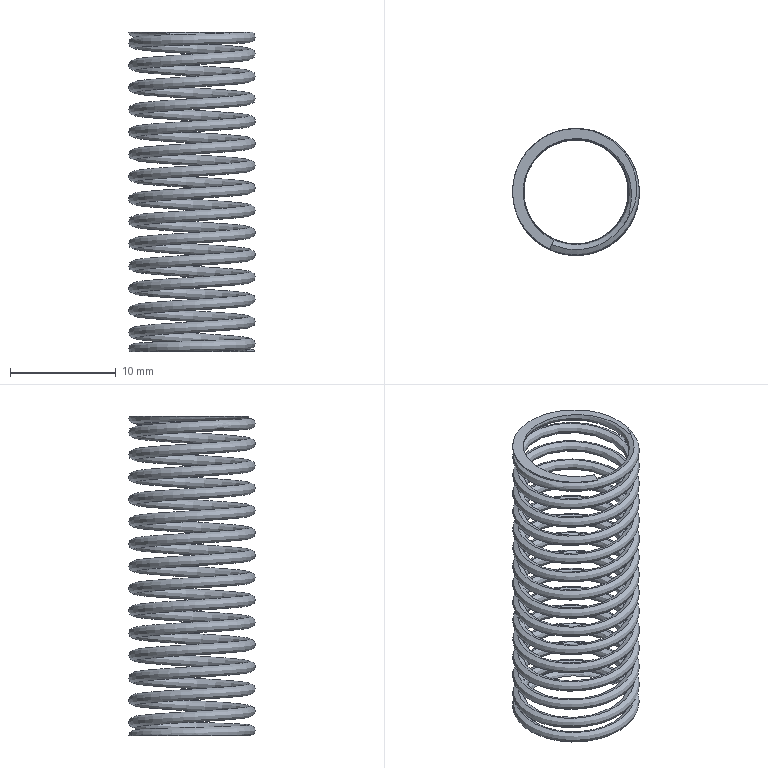Part | NX | features BREP 1 | 1 solid | 6 faces | volume 411.355 mm3 | plane 4 | spline 2